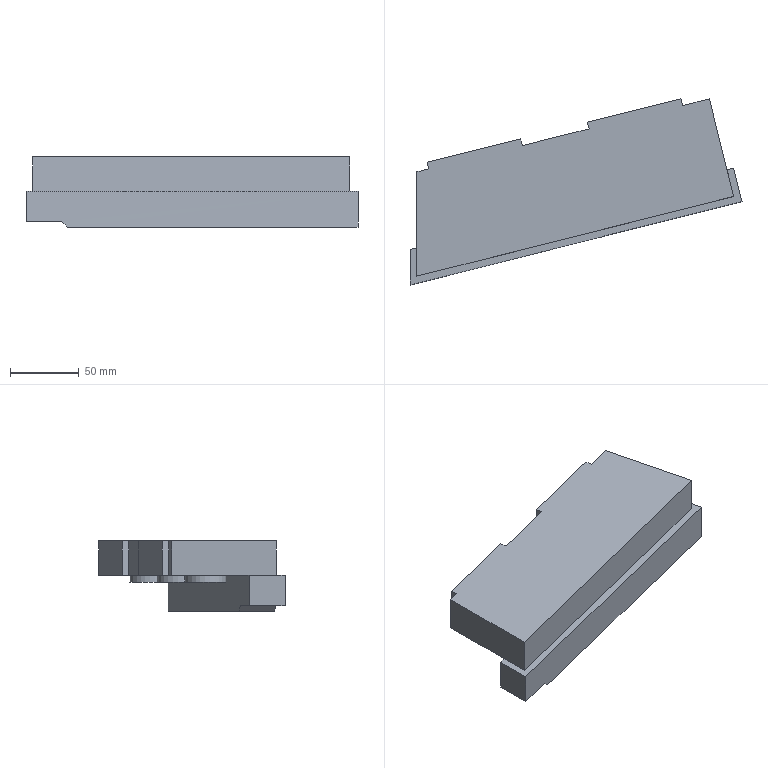Part | NX | features solid 2 | 1 solid | 32 faces | box 241.149 x 135.184 x 51 mm | volume 609918 mm3 | plane 24 | cylinder 5 | spline 3 | commonest cylinder face diameters 30 x5
STEP:
#1=CARTESIAN_POINT('',(-290.,474.207,-2.));
#2=VERTEX_POINT('',#1);
#3=CARTESIAN_POINT('',(-290.,499.994,-2.));
#4=VERTEX_POINT('',#3);
#5=CARTESIAN_POINT('',(-290.,600.,-2.));
#6=DIRECTION('',(0.,1.,0.));
#7=VECTOR('',#6,1000.);
#8=LINE('',#5,#7);
#9=EDGE_CURVE('',#2,#4,#8,.T.);
#10=ORIENTED_EDGE('',*,*,#9,.F.);
#11=CARTESIAN_POINT('',(-290.,474.207,20.));
#12=VERTEX_POINT('',#11);
#13=CARTESIAN_POINT('',(-290.,474.207,7.));
#14=DIRECTION('',(0.,0.,-1.));
#15=VECTOR('',#14,1000.);
#16=LINE('',#13,#15);
#17=EDGE_CURVE('',#2,#12,#16,.F.);
#18=ORIENTED_EDGE('',*,*,#17,.T.);
#19=CARTESIAN_POINT('',(-290.,499.994,20.));
#20=VERTEX_POINT('',#19);
#21=CARTESIAN_POINT('',(-290.,359.461,20.));
#22=DIRECTION('',(0.,-1.,0.));
#23=VECTOR('',#22,1000.);
#24=LINE('',#21,#23);
#25=EDGE_CURVE('',#12,#20,#24,.F.);
#26=ORIENTED_EDGE('',*,*,#25,.T.);
#27=CARTESIAN_POINT('',(-290.,499.994,7.));
#28=DIRECTION('',(0.,0.,1.));
#29=VECTOR('',#28,1000.);
#30=LINE('',#27,#29);
#31=EDGE_CURVE('',#20,#4,#30,.F.);
#32=ORIENTED_EDGE('',*,*,#31,.T.);
#33=EDGE_LOOP('',(#10,#18,#26,#32));
#34=FACE_BOUND('',#33,.T.);
#35=CARTESIAN_POINT('',(-290.,600.,0.));
#36=DIRECTION('',(-1.,0.,0.));
#37=DIRECTION('',(0.,0.,1.));
#38=AXIS2_PLACEMENT_3D('',#35,#36,#37);
#39=PLANE('',#38);
#40=ADVANCED_FACE('',(#34),#39,.T.);
#41=CARTESIAN_POINT('',(-192.908,552.089,20.));
#42=VERTEX_POINT('',#41);
#43=CARTESIAN_POINT('',(-177.908,552.089,20.));
#44=DIRECTION('',(0.,0.,-1.));
#45=DIRECTION('',(-1.,0.,0.));
#46=AXIS2_PLACEMENT_3D('',#43,#44,#45);
#47=CIRCLE('',#46,15.);
#48=EDGE_CURVE('',#42,#42,#47,.T.);
#49=ORIENTED_EDGE('',*,*,#48,.F.);
#50=EDGE_LOOP('',(#49));
#51=FACE_BOUND('',#50,.T.);
#52=CARTESIAN_POINT('',(-242.908,552.089,20.));
#53=VERTEX_POINT('',#52);
#54=CARTESIAN_POINT('',(-227.908,552.089,20.));
#55=DIRECTION('',(0.,0.,-1.));
#56=DIRECTION('',(-1.,0.,0.));
#57=AXIS2_PLACEMENT_3D('',#54,#55,#56);
#58=CIRCLE('',#57,15.);
#59=EDGE_CURVE('',#53,#53,#58,.T.);
#60=ORIENTED_EDGE('',*,*,#59,.F.);
#61=EDGE_LOOP('',(#60));
#62=FACE_BOUND('',#61,.T.);
#63=CARTESIAN_POINT('',(-272.908,532.089,20.));
#64=VERTEX_POINT('',#63);
#65=CARTESIAN_POINT('',(-257.908,532.089,20.));
#66=DIRECTION('',(0.,0.,-1.));
#67=DIRECTION('',(-1.,0.,0.));
#68=AXIS2_PLACEMENT_3D('',#65,#66,#67);
#69=CIRCLE('',#68,15.);
#70=EDGE_CURVE('',#64,#64,#69,.T.);
#71=ORIENTED_EDGE('',*,*,#70,.F.);
#72=EDGE_LOOP('',(#71));
#73=FACE_BOUND('',#72,.T.);
#74=CARTESIAN_POINT('',(-147.908,572.089,20.));
#75=VERTEX_POINT('',#74);
#76=CARTESIAN_POINT('',(-132.908,572.089,20.));
#77=DIRECTION('',(0.,0.,-1.));
#78=DIRECTION('',(-1.,0.,0.));
#79=AXIS2_PLACEMENT_3D('',#76,#77,#78);
#80=CIRCLE('',#79,15.);
#81=EDGE_CURVE('',#75,#75,#80,.T.);
#82=ORIENTED_EDGE('',*,*,#81,.F.);
#83=EDGE_LOOP('',(#82));
#84=FACE_BOUND('',#83,.T.);
#85=CARTESIAN_POINT('',(-112.908,572.089,20.));
#86=VERTEX_POINT('',#85);
#87=CARTESIAN_POINT('',(-97.908,572.089,20.));
#88=DIRECTION('',(0.,0.,-1.));
#89=DIRECTION('',(-1.,0.,0.));
#90=AXIS2_PLACEMENT_3D('',#87,#88,#89);
#91=CIRCLE('',#90,15.);
#92=EDGE_CURVE('',#86,#86,#91,.T.);
#93=ORIENTED_EDGE('',*,*,#92,.F.);
#94=EDGE_LOOP('',(#93));
#95=FACE_BOUND('',#94,.T.);
#96=CARTESIAN_POINT('',(-285.,501.256,20.));
#97=VERTEX_POINT('',#96);
#98=CARTESIAN_POINT('',(-59.748,557.921,20.));
#99=VERTEX_POINT('',#98);
#100=CARTESIAN_POINT('',(-285.,501.256,20.));
#101=CARTESIAN_POINT('',(-266.232,505.989,20.));
#102=CARTESIAN_POINT('',(-228.669,515.351,20.));
#103=CARTESIAN_POINT('',(-153.588,534.251,20.));
#104=CARTESIAN_POINT('',(-97.288,548.469,20.));
#105=CARTESIAN_POINT('',(-59.748,557.921,20.));
#106=B_SPLINE_CURVE_WITH_KNOTS('',3,(#100,#101,#102,#103,#104,#105),.UNSPECIFIED.,.F.,.F.,(4,1,1,4),(0.4597,0.5177,0.5758,0.6919),.UNSPECIFIED.);
#107=EDGE_CURVE('',#97,#99,#106,.T.);
#108=ORIENTED_EDGE('',*,*,#107,.F.);
#109=CARTESIAN_POINT('',(-285.,556.415,20.));
#110=VERTEX_POINT('',#109);
#111=CARTESIAN_POINT('',(-285.,482.459,20.));
#112=DIRECTION('',(0.,-1.,0.));
#113=VECTOR('',#112,1000.);
#114=LINE('',#111,#113);
#115=EDGE_CURVE('',#97,#110,#114,.F.);
#116=ORIENTED_EDGE('',*,*,#115,.T.);
#117=CARTESIAN_POINT('',(-276.34,558.574,20.));
#118=VERTEX_POINT('',#117);
#119=CARTESIAN_POINT('',(-334.558,544.059,20.));
#120=DIRECTION('',(-0.9703,-0.2419,0.));
#121=VECTOR('',#120,1000.);
#122=LINE('',#119,#121);
#123=EDGE_CURVE('',#110,#118,#122,.F.);
#124=ORIENTED_EDGE('',*,*,#123,.T.);
#125=CARTESIAN_POINT('',(-277.549,563.426,20.));
#126=VERTEX_POINT('',#125);
#127=CARTESIAN_POINT('',(-246.318,438.164,20.));
#128=DIRECTION('',(0.2419,-0.9703,0.));
#129=VECTOR('',#128,1000.);
#130=LINE('',#127,#129);
#131=EDGE_CURVE('',#118,#126,#130,.F.);
#132=ORIENTED_EDGE('',*,*,#131,.T.);
#133=CARTESIAN_POINT('',(-209.629,580.36,20.));
#134=VERTEX_POINT('',#133);
#135=CARTESIAN_POINT('',(-335.767,548.911,20.));
#136=DIRECTION('',(0.9703,0.2419,0.));
#137=VECTOR('',#136,1000.);
#138=LINE('',#135,#137);
#139=EDGE_CURVE('',#126,#134,#138,.T.);
#140=ORIENTED_EDGE('',*,*,#139,.T.);
#141=CARTESIAN_POINT('',(-208.419,575.509,20.));
#142=VERTEX_POINT('',#141);
#143=CARTESIAN_POINT('',(-178.397,455.098,20.));
#144=DIRECTION('',(0.2419,-0.9703,0.));
#145=VECTOR('',#144,1000.);
#146=LINE('',#143,#145);
#147=EDGE_CURVE('',#142,#134,#146,.F.);
#148=ORIENTED_EDGE('',*,*,#147,.F.);
#149=CARTESIAN_POINT('',(-159.904,587.605,20.));
#150=VERTEX_POINT('',#149);
#151=CARTESIAN_POINT('',(-334.558,544.059,20.));
#152=DIRECTION('',(-0.9703,-0.2419,0.));
#153=VECTOR('',#152,1000.);
#154=LINE('',#151,#153);
#155=EDGE_CURVE('',#142,#150,#154,.F.);
#156=ORIENTED_EDGE('',*,*,#155,.T.);
#157=CARTESIAN_POINT('',(-161.114,592.457,20.));
#158=VERTEX_POINT('',#157);
#159=CARTESIAN_POINT('',(-159.904,587.605,20.));
#160=DIRECTION('',(-0.2419,0.9703,0.));
#161=VECTOR('',#160,1000.);
#162=LINE('',#159,#161);
#163=EDGE_CURVE('',#150,#158,#162,.T.);
#164=ORIENTED_EDGE('',*,*,#163,.T.);
#165=CARTESIAN_POINT('',(-93.193,609.391,20.));
#166=VERTEX_POINT('',#165);
#167=CARTESIAN_POINT('',(-132.005,599.714,20.));
#168=DIRECTION('',(0.9703,0.2419,0.));
#169=VECTOR('',#168,1000.);
#170=LINE('',#167,#169);
#171=EDGE_CURVE('',#158,#166,#170,.T.);
#172=ORIENTED_EDGE('',*,*,#171,.T.);
#173=CARTESIAN_POINT('',(-91.984,604.54,20.));
#174=VERTEX_POINT('',#173);
#175=CARTESIAN_POINT('',(-91.984,604.54,20.));
#176=DIRECTION('',(-0.2419,0.9703,0.));
#177=VECTOR('',#176,1000.);
#178=LINE('',#175,#177);
#179=EDGE_CURVE('',#174,#166,#178,.T.);
#180=ORIENTED_EDGE('',*,*,#179,.F.);
#181=CARTESIAN_POINT('',(-72.578,609.378,20.));
#182=VERTEX_POINT('',#181);
#183=CARTESIAN_POINT('',(-334.558,544.059,20.));
#184=DIRECTION('',(-0.9703,-0.2419,0.));
#185=VECTOR('',#184,1000.);
#186=LINE('',#183,#185);
#187=EDGE_CURVE('',#174,#182,#186,.F.);
#188=ORIENTED_EDGE('',*,*,#187,.T.);
#189=CARTESIAN_POINT('',(-54.912,538.526,20.));
#190=DIRECTION('',(0.2419,-0.9703,0.));
#191=VECTOR('',#190,1000.);
#192=LINE('',#189,#191);
#193=EDGE_CURVE('',#99,#182,#192,.F.);
#194=ORIENTED_EDGE('',*,*,#193,.F.);
#195=EDGE_LOOP('',(#108,#116,#124,#132,#140,#148,#156,#164,#172,#180,#188,#194));
#196=FACE_BOUND('',#195,.T.);
#197=CARTESIAN_POINT('',(-561.977,359.461,20.));
#198=DIRECTION('',(0.,0.,-1.));
#199=DIRECTION('',(-1.,0.,0.));
#200=AXIS2_PLACEMENT_3D('',#197,#198,#199);
#201=PLANE('',#200);
#202=ADVANCED_FACE('',(#51,#62,#73,#84,#95,#196),#201,.T.);
#203=CARTESIAN_POINT('',(-285.,480.629,45.));
#204=VERTEX_POINT('',#203);
#205=CARTESIAN_POINT('',(-285.,556.415,45.));
#206=VERTEX_POINT('',#205);
#207=CARTESIAN_POINT('',(-285.,-794.984,45.));
#208=DIRECTION('',(0.,1.,0.));
#209=VECTOR('',#208,1000.);
#210=LINE('',#207,#209);
#211=EDGE_CURVE('',#204,#206,#210,.T.);
#212=ORIENTED_EDGE('',*,*,#211,.F.);
#213=CARTESIAN_POINT('',(-54.91,538.515,45.));
#214=VERTEX_POINT('',#213);
#215=CARTESIAN_POINT('',(-285.,480.629,45.));
#216=CARTESIAN_POINT('',(-265.83,485.471,45.));
#217=CARTESIAN_POINT('',(-227.462,495.038,45.));
#218=CARTESIAN_POINT('',(-150.765,514.332,45.));
#219=CARTESIAN_POINT('',(-93.256,528.86,45.));
#220=CARTESIAN_POINT('',(-54.91,538.515,45.));
#221=B_SPLINE_CURVE_WITH_KNOTS('',3,(#215,#216,#217,#218,#219,#220),.UNSPECIFIED.,.F.,.F.,(4,1,1,4),(0.02774,0.08706,0.1464,0.265),.UNSPECIFIED.);
#222=EDGE_CURVE('',#204,#214,#221,.T.);
#223=ORIENTED_EDGE('',*,*,#222,.T.);
#224=CARTESIAN_POINT('',(-72.578,609.378,45.));
#225=VERTEX_POINT('',#224);
#226=CARTESIAN_POINT('',(-54.912,538.526,45.));
#227=DIRECTION('',(-0.2419,0.9703,0.));
#228=VECTOR('',#227,1000.);
#229=LINE('',#226,#228);
#230=EDGE_CURVE('',#214,#225,#229,.T.);
#231=ORIENTED_EDGE('',*,*,#230,.T.);
#232=CARTESIAN_POINT('',(-91.984,604.54,45.));
#233=VERTEX_POINT('',#232);
#234=CARTESIAN_POINT('',(-334.558,544.059,45.));
#235=DIRECTION('',(0.9703,0.2419,0.));
#236=VECTOR('',#235,1000.);
#237=LINE('',#234,#236);
#238=EDGE_CURVE('',#233,#225,#237,.T.);
#239=ORIENTED_EDGE('',*,*,#238,.F.);
#240=CARTESIAN_POINT('',(-93.193,609.391,45.));
#241=VERTEX_POINT('',#240);
#242=CARTESIAN_POINT('',(-91.984,604.54,45.));
#243=DIRECTION('',(-0.2419,0.9703,0.));
#244=VECTOR('',#243,1000.);
#245=LINE('',#242,#244);
#246=EDGE_CURVE('',#233,#241,#245,.T.);
#247=ORIENTED_EDGE('',*,*,#246,.T.);
#248=CARTESIAN_POINT('',(-161.114,592.457,45.));
#249=VERTEX_POINT('',#248);
#250=CARTESIAN_POINT('',(-132.005,599.714,45.));
#251=DIRECTION('',(0.9703,0.2419,0.));
#252=VECTOR('',#251,1000.);
#253=LINE('',#250,#252);
#254=EDGE_CURVE('',#249,#241,#253,.T.);
#255=ORIENTED_EDGE('',*,*,#254,.F.);
#256=CARTESIAN_POINT('',(-159.904,587.605,45.));
#257=VERTEX_POINT('',#256);
#258=CARTESIAN_POINT('',(-159.904,587.605,45.));
#259=DIRECTION('',(-0.2419,0.9703,0.));
#260=VECTOR('',#259,1000.);
#261=LINE('',#258,#260);
#262=EDGE_CURVE('',#257,#249,#261,.T.);
#263=ORIENTED_EDGE('',*,*,#262,.F.);
#264=CARTESIAN_POINT('',(-208.419,575.509,45.));
#265=VERTEX_POINT('',#264);
#266=CARTESIAN_POINT('',(-334.558,544.059,45.));
#267=DIRECTION('',(0.9703,0.2419,0.));
#268=VECTOR('',#267,1000.);
#269=LINE('',#266,#268);
#270=EDGE_CURVE('',#265,#257,#269,.T.);
#271=ORIENTED_EDGE('',*,*,#270,.F.);
#272=CARTESIAN_POINT('',(-209.629,580.36,45.));
#273=VERTEX_POINT('',#272);
#274=CARTESIAN_POINT('',(120.792,-744.886,45.));
#275=DIRECTION('',(-0.2419,0.9703,0.));
#276=VECTOR('',#275,1000.);
#277=LINE('',#274,#276);
#278=EDGE_CURVE('',#265,#273,#277,.T.);
#279=ORIENTED_EDGE('',*,*,#278,.T.);
#280=CARTESIAN_POINT('',(-277.549,563.426,45.));
#281=VERTEX_POINT('',#280);
#282=CARTESIAN_POINT('',(-335.767,548.911,45.));
#283=DIRECTION('',(0.9703,0.2419,0.));
#284=VECTOR('',#283,1000.);
#285=LINE('',#282,#284);
#286=EDGE_CURVE('',#281,#273,#285,.T.);
#287=ORIENTED_EDGE('',*,*,#286,.F.);
#288=CARTESIAN_POINT('',(-276.34,558.574,45.));
#289=VERTEX_POINT('',#288);
#290=CARTESIAN_POINT('',(52.872,-761.821,45.));
#291=DIRECTION('',(-0.2419,0.9703,0.));
#292=VECTOR('',#291,1000.);
#293=LINE('',#290,#292);
#294=EDGE_CURVE('',#289,#281,#293,.T.);
#295=ORIENTED_EDGE('',*,*,#294,.F.);
#296=CARTESIAN_POINT('',(-334.558,544.059,45.));
#297=DIRECTION('',(0.9703,0.2419,0.));
#298=VECTOR('',#297,1000.);
#299=LINE('',#296,#298);
#300=EDGE_CURVE('',#206,#289,#299,.T.);
#301=ORIENTED_EDGE('',*,*,#300,.F.);
#302=EDGE_LOOP('',(#212,#223,#231,#239,#247,#255,#263,#271,#279,#287,#295,#301));
#303=FACE_BOUND('',#302,.T.);
#304=CARTESIAN_POINT('',(-80.139,-794.984,45.));
#305=DIRECTION('',(0.,0.,1.));
#306=DIRECTION('',(1.,0.,0.));
#307=AXIS2_PLACEMENT_3D('',#304,#305,#306);
#308=PLANE('',#307);
#309=ADVANCED_FACE('',(#303),#308,.T.);
#310=CARTESIAN_POINT('',(-260.,481.763,-6.));
#311=VERTEX_POINT('',#310);
#312=CARTESIAN_POINT('',(-48.851,534.884,-6.));
#313=VERTEX_POINT('',#312);
#314=CARTESIAN_POINT('',(-48.851,534.884,-6.));
#315=CARTESIAN_POINT('',(-84.041,526.025,-6.));
#316=CARTESIAN_POINT('',(-154.403,508.24,-6.));
#317=CARTESIAN_POINT('',(-224.801,490.59,-6.));
#318=CARTESIAN_POINT('',(-260.,481.763,-6.));
#319=B_SPLINE_CURVE_WITH_KNOTS('',3,(#314,#315,#316,#317,#318),.UNSPECIFIED.,.F.,.F.,(4,1,4),(0.4841,0.5929,0.7018),.UNSPECIFIED.);
#320=EDGE_CURVE('',#311,#313,#319,.F.);
#321=ORIENTED_EDGE('',*,*,#320,.F.);
#322=CARTESIAN_POINT('',(-260.,507.536,-6.));
#323=VERTEX_POINT('',#322);
#324=CARTESIAN_POINT('',(-260.,-794.984,-6.));
#325=DIRECTION('',(0.,1.,0.));
#326=VECTOR('',#325,1000.);
#327=LINE('',#324,#326);
#328=EDGE_CURVE('',#311,#323,#327,.T.);
#329=ORIENTED_EDGE('',*,*,#328,.T.);
#330=CARTESIAN_POINT('',(-54.899,559.142,-6.));
#331=VERTEX_POINT('',#330);
#332=CARTESIAN_POINT('',(-260.,507.536,-6.));
#333=CARTESIAN_POINT('',(-191.614,524.661,-6.));
#334=CARTESIAN_POINT('',(-123.264,541.93,-6.));
#335=CARTESIAN_POINT('',(-54.899,559.142,-6.));
#336=B_SPLINE_CURVE_WITH_KNOTS('',3,(#332,#333,#334,#335),.UNSPECIFIED.,.F.,.F.,(4,4),(0.4856,0.6971),.UNSPECIFIED.);
#337=EDGE_CURVE('',#323,#331,#336,.T.);
#338=ORIENTED_EDGE('',*,*,#337,.T.);
#339=CARTESIAN_POINT('',(563.408,-1920.754,-6.));
#340=DIRECTION('',(-0.2419,0.9703,0.));
#341=VECTOR('',#340,1000.);
#342=LINE('',#339,#341);
#343=EDGE_CURVE('',#313,#331,#342,.T.);
#344=ORIENTED_EDGE('',*,*,#343,.F.);
#345=EDGE_LOOP('',(#321,#329,#338,#344));
#346=FACE_BOUND('',#345,.T.);
#347=CARTESIAN_POINT('',(-80.139,-794.984,-6.));
#348=DIRECTION('',(0.,0.,1.));
#349=DIRECTION('',(1.,0.,0.));
#350=AXIS2_PLACEMENT_3D('',#347,#348,#349);
#351=PLANE('',#350);
#352=ADVANCED_FACE('',(#346),#351,.F.);
#353=CARTESIAN_POINT('',(-264.,480.76,-2.));
#354=VERTEX_POINT('',#353);
#355=CARTESIAN_POINT('',(-290.,474.207,-2.));
#356=CARTESIAN_POINT('',(-281.336,476.401,-2.));
#357=CARTESIAN_POINT('',(-272.669,478.584,-2.));
#358=CARTESIAN_POINT('',(-264.,480.76,-2.));
#359=B_SPLINE_CURVE_WITH_KNOTS('',3,(#355,#356,#357,#358),.UNSPECIFIED.,.F.,.F.,(4,4),(0.1598,0.1865),.UNSPECIFIED.);
#360=EDGE_CURVE('',#2,#354,#359,.T.);
#361=ORIENTED_EDGE('',*,*,#360,.T.);
#362=CARTESIAN_POINT('',(-264.,480.76,-2.));
#363=CARTESIAN_POINT('',(-262.667,481.095,-3.333));
#364=CARTESIAN_POINT('',(-261.333,481.429,-4.667));
#365=CARTESIAN_POINT('',(-260.,481.763,-6.));
#366=B_SPLINE_CURVE_WITH_KNOTS('',3,(#362,#363,#364,#365),.UNSPECIFIED.,.F.,.F.,(4,4),(0.,0.005745),.UNSPECIFIED.);
#367=EDGE_CURVE('',#354,#311,#366,.T.);
#368=ORIENTED_EDGE('',*,*,#367,.T.);
#369=ORIENTED_EDGE('',*,*,#320,.T.);
#370=CARTESIAN_POINT('',(-48.851,534.884,20.));
#371=VERTEX_POINT('',#370);
#372=CARTESIAN_POINT('',(-48.851,534.884,30.));
#373=DIRECTION('',(0.,0.,-1.));
#374=VECTOR('',#373,1000.);
#375=LINE('',#372,#374);
#376=EDGE_CURVE('',#371,#313,#375,.T.);
#377=ORIENTED_EDGE('',*,*,#376,.F.);
#378=CARTESIAN_POINT('',(-48.851,534.884,20.));
#379=CARTESIAN_POINT('',(-89.041,524.766,20.));
#380=CARTESIAN_POINT('',(-149.312,509.537,20.));
#381=CARTESIAN_POINT('',(-229.699,489.326,20.));
#382=CARTESIAN_POINT('',(-269.912,479.293,20.));
#383=CARTESIAN_POINT('',(-290.,474.207,20.));
#384=B_SPLINE_CURVE_WITH_KNOTS('',3,(#378,#379,#380,#381,#382,#383),.UNSPECIFIED.,.F.,.F.,(4,1,1,4),(0.4669,0.5913,0.6534,0.7156),.UNSPECIFIED.);
#385=EDGE_CURVE('',#12,#371,#384,.F.);
#386=ORIENTED_EDGE('',*,*,#385,.F.);
#387=ORIENTED_EDGE('',*,*,#17,.F.);
#388=EDGE_LOOP('',(#361,#368,#369,#377,#386,#387));
#389=FACE_BOUND('',#388,.T.);
#390=CARTESIAN_POINT('',(-290.,474.207,20.));
#391=CARTESIAN_POINT('',(-290.,474.207,-6.));
#392=CARTESIAN_POINT('',(-269.911,479.293,20.));
#393=CARTESIAN_POINT('',(-269.911,479.293,-6.));
#394=CARTESIAN_POINT('',(-229.7,489.326,20.));
#395=CARTESIAN_POINT('',(-229.7,489.326,-6.));
#396=CARTESIAN_POINT('',(-149.313,509.536,20.));
#397=CARTESIAN_POINT('',(-149.313,509.536,-6.));
#398=CARTESIAN_POINT('',(-89.041,524.766,20.));
#399=CARTESIAN_POINT('',(-89.041,524.766,-6.));
#400=CARTESIAN_POINT('',(-48.851,534.884,20.));
#401=CARTESIAN_POINT('',(-48.851,534.884,-6.));
#402=B_SPLINE_SURFACE_WITH_KNOTS('',3,1,((#390,#391),(#392,#393),(#394,#395),(#396,#397),(#398,#399),(#400,#401)),.SURF_OF_LINEAR_EXTRUSION.,.F.,.F.,.F.,(4,1,1,4),(2,2),(0.5601,0.6132,0.6663,0.7724),(0.,1.),.UNSPECIFIED.);
#403=ADVANCED_FACE('',(#389),#402,.F.);
#404=CARTESIAN_POINT('',(-285.,480.629,20.));
#405=VERTEX_POINT('',#404);
#406=CARTESIAN_POINT('',(-54.91,538.515,20.));
#407=VERTEX_POINT('',#406);
#408=CARTESIAN_POINT('',(-285.,480.629,20.));
#409=CARTESIAN_POINT('',(-265.83,485.471,20.));
#410=CARTESIAN_POINT('',(-227.462,495.038,20.));
#411=CARTESIAN_POINT('',(-150.765,514.332,20.));
#412=CARTESIAN_POINT('',(-93.256,528.86,20.));
#413=CARTESIAN_POINT('',(-54.91,538.515,20.));
#414=B_SPLINE_CURVE_WITH_KNOTS('',3,(#408,#409,#410,#411,#412,#413),.UNSPECIFIED.,.F.,.F.,(4,1,1,4),(1.119,1.178,1.237,1.356),.UNSPECIFIED.);
#415=EDGE_CURVE('',#405,#407,#414,.T.);
#416=ORIENTED_EDGE('',*,*,#415,.F.);
#417=CARTESIAN_POINT('',(-285.,482.459,20.));
#418=DIRECTION('',(0.,-1.,0.));
#419=VECTOR('',#418,1000.);
#420=LINE('',#417,#419);
#421=EDGE_CURVE('',#405,#97,#420,.F.);
#422=ORIENTED_EDGE('',*,*,#421,.T.);
#423=CARTESIAN_POINT('',(-290.,499.994,20.));
#424=CARTESIAN_POINT('',(-288.333,500.415,20.));
#425=CARTESIAN_POINT('',(-286.667,500.836,20.));
#426=CARTESIAN_POINT('',(-285.,501.256,20.));
#427=B_SPLINE_CURVE_WITH_KNOTS('',3,(#423,#424,#425,#426),.UNSPECIFIED.,.F.,.F.,(4,4),(0.4545,0.4597),.UNSPECIFIED.);
#428=EDGE_CURVE('',#20,#97,#427,.T.);
#429=ORIENTED_EDGE('',*,*,#428,.F.);
#430=ORIENTED_EDGE('',*,*,#25,.F.);
#431=ORIENTED_EDGE('',*,*,#385,.T.);
#432=CARTESIAN_POINT('',(-54.899,559.142,20.));
#433=VERTEX_POINT('',#432);
#434=CARTESIAN_POINT('',(-48.691,534.243,20.));
#435=DIRECTION('',(0.2419,-0.9703,0.));
#436=VECTOR('',#435,1000.);
#437=LINE('',#434,#436);
#438=EDGE_CURVE('',#371,#433,#437,.F.);
#439=ORIENTED_EDGE('',*,*,#438,.T.);
#440=CARTESIAN_POINT('',(-54.899,559.142,20.));
#441=CARTESIAN_POINT('',(-56.516,558.735,20.));
#442=CARTESIAN_POINT('',(-58.132,558.328,20.));
#443=CARTESIAN_POINT('',(-59.748,557.921,20.));
#444=B_SPLINE_CURVE_WITH_KNOTS('',3,(#440,#441,#442,#443),.UNSPECIFIED.,.F.,.F.,(4,4),(0.,0.005),.UNSPECIFIED.);
#445=EDGE_CURVE('',#99,#433,#444,.F.);
#446=ORIENTED_EDGE('',*,*,#445,.F.);
#447=CARTESIAN_POINT('',(-53.543,533.033,20.));
#448=DIRECTION('',(0.2419,-0.9703,0.));
#449=VECTOR('',#448,1000.);
#450=LINE('',#447,#449);
#451=EDGE_CURVE('',#407,#99,#450,.F.);
#452=ORIENTED_EDGE('',*,*,#451,.F.);
#453=EDGE_LOOP('',(#416,#422,#429,#430,#431,#439,#446,#452));
#454=FACE_BOUND('',#453,.T.);
#455=CARTESIAN_POINT('',(-561.977,359.461,20.));
#456=DIRECTION('',(0.,0.,1.));
#457=DIRECTION('',(1.,0.,0.));
#458=AXIS2_PLACEMENT_3D('',#455,#456,#457);
#459=PLANE('',#458);
#460=ADVANCED_FACE('',(#454),#459,.T.);
#461=CARTESIAN_POINT('',(-285.,556.415,70.));
#462=DIRECTION('',(0.,0.,-1.));
#463=VECTOR('',#462,1000.);
#464=LINE('',#461,#463);
#465=EDGE_CURVE('',#206,#110,#464,.T.);
#466=ORIENTED_EDGE('',*,*,#465,.F.);
#467=ORIENTED_EDGE('',*,*,#300,.T.);
#468=CARTESIAN_POINT('',(-276.34,558.574,70.));
#469=DIRECTION('',(0.,0.,-1.));
#470=VECTOR('',#469,1000.);
#471=LINE('',#468,#470);
#472=EDGE_CURVE('',#289,#118,#471,.T.);
#473=ORIENTED_EDGE('',*,*,#472,.T.);
#474=ORIENTED_EDGE('',*,*,#123,.F.);
#475=EDGE_LOOP('',(#466,#467,#473,#474));
#476=FACE_BOUND('',#475,.T.);
#477=CARTESIAN_POINT('',(-334.558,544.059,70.));
#478=DIRECTION('',(-0.2419,0.9703,0.));
#479=DIRECTION('',(-0.9703,-0.2419,0.));
#480=AXIS2_PLACEMENT_3D('',#477,#478,#479);
#481=PLANE('',#480);
#482=ADVANCED_FACE('',(#476),#481,.T.);
#483=ORIENTED_EDGE('',*,*,#222,.F.);
#484=CARTESIAN_POINT('',(-285.,480.629,32.5));
#485=DIRECTION('',(0.,0.,-1.));
#486=VECTOR('',#485,1000.);
#487=LINE('',#484,#486);
#488=EDGE_CURVE('',#204,#405,#487,.T.);
#489=ORIENTED_EDGE('',*,*,#488,.T.);
#490=ORIENTED_EDGE('',*,*,#415,.T.);
#491=CARTESIAN_POINT('',(-54.91,538.515,42.5));
#492=DIRECTION('',(0.,0.,-1.));
#493=VECTOR('',#492,1000.);
#494=LINE('',#491,#493);
#495=EDGE_CURVE('',#214,#407,#494,.T.);
#496=ORIENTED_EDGE('',*,*,#495,.F.);
#497=EDGE_LOOP('',(#483,#489,#490,#496));
#498=FACE_BOUND('',#497,.T.);
#499=CARTESIAN_POINT('',(-285.,480.629,45.));
#500=CARTESIAN_POINT('',(-285.,480.629,20.));
#501=CARTESIAN_POINT('',(-265.823,485.473,45.));
#502=CARTESIAN_POINT('',(-265.823,485.473,20.));
#503=CARTESIAN_POINT('',(-227.448,495.042,45.));
#504=CARTESIAN_POINT('',(-227.448,495.042,20.));
#505=CARTESIAN_POINT('',(-150.771,514.33,45.));
#506=CARTESIAN_POINT('',(-150.771,514.33,20.));
#507=CARTESIAN_POINT('',(-93.256,528.86,45.));
#508=CARTESIAN_POINT('',(-93.256,528.86,20.));
#509=CARTESIAN_POINT('',(-54.91,538.515,45.));
#510=CARTESIAN_POINT('',(-54.91,538.515,20.));
#511=B_SPLINE_SURFACE_WITH_KNOTS('',3,1,((#499,#500),(#501,#502),(#503,#504),(#505,#506),(#507,#508),(#509,#510)),.SURF_OF_LINEAR_EXTRUSION.,.F.,.F.,.F.,(4,1,1,4),(2,2),(0.1028,0.3225,0.5422,0.9815),(0.,1.),.UNSPECIFIED.);
#512=ADVANCED_FACE('',(#498),#511,.F.);
#513=ORIENTED_EDGE('',*,*,#337,.F.);
#514=CARTESIAN_POINT('',(-264.,506.534,-2.));
#515=VERTEX_POINT('',#514);
#516=CARTESIAN_POINT('',(-260.,507.536,-6.));
#517=CARTESIAN_POINT('',(-261.333,507.202,-4.667));
#518=CARTESIAN_POINT('',(-262.667,506.868,-3.333));
#519=CARTESIAN_POINT('',(-264.,506.534,-2.));
#520=B_SPLINE_CURVE_WITH_KNOTS('',3,(#516,#517,#518,#519),.UNSPECIFIED.,.F.,.F.,(4,4),(0.,0.005745),.UNSPECIFIED.);
#521=EDGE_CURVE('',#323,#515,#520,.T.);
#522=ORIENTED_EDGE('',*,*,#521,.T.);
#523=CARTESIAN_POINT('',(-264.,506.534,-2.));
#524=CARTESIAN_POINT('',(-272.669,504.362,-2.));
#525=CARTESIAN_POINT('',(-281.336,502.183,-2.));
#526=CARTESIAN_POINT('',(-290.,499.994,-2.));
#527=B_SPLINE_CURVE_WITH_KNOTS('',3,(#523,#524,#525,#526),.UNSPECIFIED.,.F.,.F.,(4,4),(0.002062,0.02887),.UNSPECIFIED.);
#528=EDGE_CURVE('',#515,#4,#527,.T.);
#529=ORIENTED_EDGE('',*,*,#528,.T.);
#530=ORIENTED_EDGE('',*,*,#31,.F.);
#531=ORIENTED_EDGE('',*,*,#428,.T.);
#532=ORIENTED_EDGE('',*,*,#107,.T.);
#533=ORIENTED_EDGE('',*,*,#445,.T.);
#534=CARTESIAN_POINT('',(-54.899,559.142,9.5));
#535=DIRECTION('',(0.,0.,1.));
#536=VECTOR('',#535,1000.);
#537=LINE('',#534,#536);
#538=EDGE_CURVE('',#331,#433,#537,.T.);
#539=ORIENTED_EDGE('',*,*,#538,.F.);
#540=EDGE_LOOP('',(#513,#522,#529,#530,#531,#532,#533,#539));
#541=FACE_BOUND('',#540,.T.);
#542=CARTESIAN_POINT('',(-290.,499.994,-6.));
#543=CARTESIAN_POINT('',(-290.,499.994,20.));
#544=CARTESIAN_POINT('',(-270.373,504.952,-6.));
#545=CARTESIAN_POINT('',(-270.373,504.952,20.));
#546=CARTESIAN_POINT('',(-231.142,514.732,-6.));
#547=CARTESIAN_POINT('',(-231.142,514.732,20.));
#548=CARTESIAN_POINT('',(-152.878,534.427,-6.));
#549=CARTESIAN_POINT('',(-152.878,534.427,20.));
#550=CARTESIAN_POINT('',(-94.078,549.278,-6.));
#551=CARTESIAN_POINT('',(-94.078,549.278,20.));
#552=CARTESIAN_POINT('',(-54.899,559.142,-6.));
#553=CARTESIAN_POINT('',(-54.899,559.142,20.));
#554=B_SPLINE_SURFACE_WITH_KNOTS('',3,1,((#542,#543),(#544,#545),(#546,#547),(#548,#549),(#550,#551),(#552,#553)),.SURF_OF_LINEAR_EXTRUSION.,.F.,.F.,.F.,(4,1,1,4),(2,2),(0.1024,0.3269,0.5513,1.),(0.,1.),.UNSPECIFIED.);
#555=ADVANCED_FACE('',(#541),#554,.F.);
#556=ORIENTED_EDGE('',*,*,#270,.T.);
#557=CARTESIAN_POINT('',(-159.904,587.605,45.));
#558=DIRECTION('',(0.,0.,1.));
#559=VECTOR('',#558,1000.);
#560=LINE('',#557,#559);
#561=EDGE_CURVE('',#257,#150,#560,.F.);
#562=ORIENTED_EDGE('',*,*,#561,.T.);
#563=ORIENTED_EDGE('',*,*,#155,.F.);
#564=CARTESIAN_POINT('',(-208.419,575.509,70.));
#565=DIRECTION('',(0.,0.,-1.));
#566=VECTOR('',#565,1000.);
#567=LINE('',#564,#566);
#568=EDGE_CURVE('',#265,#142,#567,.T.);
#569=ORIENTED_EDGE('',*,*,#568,.F.);
#570=EDGE_LOOP('',(#556,#562,#563,#569));
#571=FACE_BOUND('',#570,.T.);
#572=CARTESIAN_POINT('',(-334.558,544.059,70.));
#573=DIRECTION('',(-0.2419,0.9703,0.));
#574=DIRECTION('',(-0.9703,-0.2419,0.));
#575=AXIS2_PLACEMENT_3D('',#572,#573,#574);
#576=PLANE('',#575);
#577=ADVANCED_FACE('',(#571),#576,.T.);
#578=CARTESIAN_POINT('',(-91.984,604.54,45.));
#579=DIRECTION('',(0.,0.,-1.));
#580=VECTOR('',#579,1000.);
#581=LINE('',#578,#580);
#582=EDGE_CURVE('',#233,#174,#581,.T.);
#583=ORIENTED_EDGE('',*,*,#582,.F.);
#584=ORIENTED_EDGE('',*,*,#238,.T.);
#585=CARTESIAN_POINT('',(-72.578,609.378,70.));
#586=DIRECTION('',(0.,0.,-1.));
#587=VECTOR('',#586,1000.);
#588=LINE('',#585,#587);
#589=EDGE_CURVE('',#225,#182,#588,.T.);
#590=ORIENTED_EDGE('',*,*,#589,.T.);
#591=ORIENTED_EDGE('',*,*,#187,.F.);
#592=EDGE_LOOP('',(#583,#584,#590,#591));
#593=FACE_BOUND('',#592,.T.);
#594=CARTESIAN_POINT('',(-334.558,544.059,70.));
#595=DIRECTION('',(-0.2419,0.9703,0.));
#596=DIRECTION('',(-0.9703,-0.2419,0.));
#597=AXIS2_PLACEMENT_3D('',#594,#595,#596);
#598=PLANE('',#597);
#599=ADVANCED_FACE('',(#593),#598,.T.);
#600=ORIENTED_EDGE('',*,*,#343,.T.);
#601=ORIENTED_EDGE('',*,*,#538,.T.);
#602=ORIENTED_EDGE('',*,*,#438,.F.);
#603=ORIENTED_EDGE('',*,*,#376,.T.);
#604=EDGE_LOOP('',(#600,#601,#602,#603));
#605=FACE_BOUND('',#604,.T.);
#606=CARTESIAN_POINT('',(563.408,-1920.754,70.));
#607=DIRECTION('',(-0.9703,-0.2419,0.));
#608=DIRECTION('',(0.2419,-0.9703,0.));
#609=AXIS2_PLACEMENT_3D('',#606,#607,#608);
#610=PLANE('',#609);
#611=ADVANCED_FACE('',(#605),#610,.F.);
#612=ORIENTED_EDGE('',*,*,#451,.T.);
#613=ORIENTED_EDGE('',*,*,#193,.T.);
#614=ORIENTED_EDGE('',*,*,#589,.F.);
#615=ORIENTED_EDGE('',*,*,#230,.F.);
#616=ORIENTED_EDGE('',*,*,#495,.T.);
#617=EDGE_LOOP('',(#612,#613,#614,#615,#616));
#618=FACE_BOUND('',#617,.T.);
#619=CARTESIAN_POINT('',(-54.912,538.526,70.));
#620=DIRECTION('',(-0.9703,-0.2419,0.));
#621=DIRECTION('',(0.2419,-0.9703,0.));
#622=AXIS2_PLACEMENT_3D('',#619,#620,#621);
#623=PLANE('',#622);
#624=ADVANCED_FACE('',(#618),#623,.F.);
#625=CARTESIAN_POINT('',(-209.629,580.36,45.));
#626=DIRECTION('',(0.,0.,-1.));
#627=VECTOR('',#626,1000.);
#628=LINE('',#625,#627);
#629=EDGE_CURVE('',#273,#134,#628,.T.);
#630=ORIENTED_EDGE('',*,*,#629,.F.);
#631=ORIENTED_EDGE('',*,*,#278,.F.);
#632=ORIENTED_EDGE('',*,*,#568,.T.);
#633=ORIENTED_EDGE('',*,*,#147,.T.);
#634=EDGE_LOOP('',(#630,#631,#632,#633));
#635=FACE_BOUND('',#634,.T.);
#636=CARTESIAN_POINT('',(-208.419,575.509,45.));
#637=DIRECTION('',(0.9703,0.2419,0.));
#638=DIRECTION('',(-0.2419,0.9703,0.));
#639=AXIS2_PLACEMENT_3D('',#636,#637,#638);
#640=PLANE('',#639);
#641=ADVANCED_FACE('',(#635),#640,.T.);
#642=CARTESIAN_POINT('',(-277.549,563.426,45.));
#643=DIRECTION('',(0.,0.,-1.));
#644=VECTOR('',#643,1000.);
#645=LINE('',#642,#644);
#646=EDGE_CURVE('',#281,#126,#645,.T.);
#647=ORIENTED_EDGE('',*,*,#646,.T.);
#648=ORIENTED_EDGE('',*,*,#131,.F.);
#649=ORIENTED_EDGE('',*,*,#472,.F.);
#650=ORIENTED_EDGE('',*,*,#294,.T.);
#651=EDGE_LOOP('',(#647,#648,#649,#650));
#652=FACE_BOUND('',#651,.T.);
#653=CARTESIAN_POINT('',(-276.34,558.574,45.));
#654=DIRECTION('',(0.9703,0.2419,0.));
#655=DIRECTION('',(-0.2419,0.9703,0.));
#656=AXIS2_PLACEMENT_3D('',#653,#654,#655);
#657=PLANE('',#656);
#658=ADVANCED_FACE('',(#652),#657,.F.);
#659=ORIENTED_EDGE('',*,*,#629,.T.);
#660=ORIENTED_EDGE('',*,*,#139,.F.);
#661=ORIENTED_EDGE('',*,*,#646,.F.);
#662=ORIENTED_EDGE('',*,*,#286,.T.);
#663=EDGE_LOOP('',(#659,#660,#661,#662));
#664=FACE_BOUND('',#663,.T.);
#665=CARTESIAN_POINT('',(-335.767,548.911,45.));
#666=DIRECTION('',(0.2419,-0.9703,0.));
#667=DIRECTION('',(0.,0.,-1.));
#668=AXIS2_PLACEMENT_3D('',#665,#666,#667);
#669=PLANE('',#668);
#670=ADVANCED_FACE('',(#664),#669,.F.);
#671=CARTESIAN_POINT('',(-93.193,609.391,45.));
#672=DIRECTION('',(0.,0.,-1.));
#673=VECTOR('',#672,1000.);
#674=LINE('',#671,#673);
#675=EDGE_CURVE('',#241,#166,#674,.T.);
#676=ORIENTED_EDGE('',*,*,#675,.F.);
#677=ORIENTED_EDGE('',*,*,#246,.F.);
#678=ORIENTED_EDGE('',*,*,#582,.T.);
#679=ORIENTED_EDGE('',*,*,#179,.T.);
#680=EDGE_LOOP('',(#676,#677,#678,#679));
#681=FACE_BOUND('',#680,.T.);
#682=CARTESIAN_POINT('',(-91.984,604.54,45.));
#683=DIRECTION('',(0.9703,0.2419,0.));
#684=DIRECTION('',(-0.2419,0.9703,0.));
#685=AXIS2_PLACEMENT_3D('',#682,#683,#684);
#686=PLANE('',#685);
#687=ADVANCED_FACE('',(#681),#686,.T.);
#688=CARTESIAN_POINT('',(-161.114,592.457,45.));
#689=DIRECTION('',(0.,0.,1.));
#690=VECTOR('',#689,1000.);
#691=LINE('',#688,#690);
#692=EDGE_CURVE('',#249,#158,#691,.F.);
#693=ORIENTED_EDGE('',*,*,#692,.T.);
#694=ORIENTED_EDGE('',*,*,#163,.F.);
#695=ORIENTED_EDGE('',*,*,#561,.F.);
#696=ORIENTED_EDGE('',*,*,#262,.T.);
#697=EDGE_LOOP('',(#693,#694,#695,#696));
#698=FACE_BOUND('',#697,.T.);
#699=CARTESIAN_POINT('',(-159.904,587.605,45.));
#700=DIRECTION('',(0.9703,0.2419,0.));
#701=DIRECTION('',(-0.2419,0.9703,0.));
#702=AXIS2_PLACEMENT_3D('',#699,#700,#701);
#703=PLANE('',#702);
#704=ADVANCED_FACE('',(#698),#703,.F.);
#705=ORIENTED_EDGE('',*,*,#675,.T.);
#706=ORIENTED_EDGE('',*,*,#171,.F.);
#707=ORIENTED_EDGE('',*,*,#692,.F.);
#708=ORIENTED_EDGE('',*,*,#254,.T.);
#709=EDGE_LOOP('',(#705,#706,#707,#708));
#710=FACE_BOUND('',#709,.T.);
#711=CARTESIAN_POINT('',(-132.005,599.714,45.));
#712=DIRECTION('',(0.2419,-0.9703,0.));
#713=DIRECTION('',(0.,0.,-1.));
#714=AXIS2_PLACEMENT_3D('',#711,#712,#713);
#715=PLANE('',#714);
#716=ADVANCED_FACE('',(#710),#715,.F.);
#717=CARTESIAN_POINT('',(-117.908,572.089,15.));
#718=VERTEX_POINT('',#717);
#719=CARTESIAN_POINT('',(-132.908,572.089,15.));
#720=DIRECTION('',(0.,0.,-1.));
#721=DIRECTION('',(1.,0.,0.));
#722=AXIS2_PLACEMENT_3D('',#719,#720,#721);
#723=CIRCLE('',#722,15.);
#724=EDGE_CURVE('',#718,#718,#723,.T.);
#725=ORIENTED_EDGE('',*,*,#724,.F.);
#726=EDGE_LOOP('',(#725));
#727=FACE_BOUND('',#726,.T.);
#728=ORIENTED_EDGE('',*,*,#81,.T.);
#729=EDGE_LOOP('',(#728));
#730=FACE_BOUND('',#729,.T.);
#731=CARTESIAN_POINT('',(-132.908,572.089,15.));
#732=DIRECTION('',(0.,0.,1.));
#733=DIRECTION('',(1.,0.,0.));
#734=AXIS2_PLACEMENT_3D('',#731,#732,#733);
#735=CYLINDRICAL_SURFACE('',#734,15.);
#736=ADVANCED_FACE('',(#727,#730),#735,.T.);
#737=ORIENTED_EDGE('',*,*,#724,.T.);
#738=EDGE_LOOP('',(#737));
#739=FACE_BOUND('',#738,.T.);
#740=CARTESIAN_POINT('',(-132.908,572.089,15.));
#741=DIRECTION('',(0.,0.,-1.));
#742=DIRECTION('',(-1.,0.,0.));
#743=AXIS2_PLACEMENT_3D('',#740,#741,#742);
#744=PLANE('',#743);
#745=ADVANCED_FACE('',(#739),#744,.T.);
#746=CARTESIAN_POINT('',(-82.908,572.089,15.));
#747=VERTEX_POINT('',#746);
#748=CARTESIAN_POINT('',(-97.908,572.089,15.));
#749=DIRECTION('',(0.,0.,-1.));
#750=DIRECTION('',(1.,0.,0.));
#751=AXIS2_PLACEMENT_3D('',#748,#749,#750);
#752=CIRCLE('',#751,15.);
#753=EDGE_CURVE('',#747,#747,#752,.T.);
#754=ORIENTED_EDGE('',*,*,#753,.F.);
#755=EDGE_LOOP('',(#754));
#756=FACE_BOUND('',#755,.T.);
#757=ORIENTED_EDGE('',*,*,#92,.T.);
#758=EDGE_LOOP('',(#757));
#759=FACE_BOUND('',#758,.T.);
#760=CARTESIAN_POINT('',(-97.908,572.089,15.));
#761=DIRECTION('',(0.,0.,1.));
#762=DIRECTION('',(1.,0.,0.));
#763=AXIS2_PLACEMENT_3D('',#760,#761,#762);
#764=CYLINDRICAL_SURFACE('',#763,15.);
#765=ADVANCED_FACE('',(#756,#759),#764,.T.);
#766=ORIENTED_EDGE('',*,*,#753,.T.);
#767=EDGE_LOOP('',(#766));
#768=FACE_BOUND('',#767,.T.);
#769=CARTESIAN_POINT('',(-97.908,572.089,15.));
#770=DIRECTION('',(0.,0.,-1.));
#771=DIRECTION('',(-1.,0.,0.));
#772=AXIS2_PLACEMENT_3D('',#769,#770,#771);
#773=PLANE('',#772);
#774=ADVANCED_FACE('',(#768),#773,.T.);
#775=ORIENTED_EDGE('',*,*,#465,.T.);
#776=ORIENTED_EDGE('',*,*,#115,.F.);
#777=ORIENTED_EDGE('',*,*,#421,.F.);
#778=ORIENTED_EDGE('',*,*,#488,.F.);
#779=ORIENTED_EDGE('',*,*,#211,.T.);
#780=EDGE_LOOP('',(#775,#776,#777,#778,#779));
#781=FACE_BOUND('',#780,.T.);
#782=CARTESIAN_POINT('',(-285.,482.459,20.));
#783=DIRECTION('',(1.,0.,0.));
#784=DIRECTION('',(0.,0.,-1.));
#785=AXIS2_PLACEMENT_3D('',#782,#783,#784);
#786=PLANE('',#785);
#787=ADVANCED_FACE('',(#781),#786,.F.);
#788=ORIENTED_EDGE('',*,*,#528,.F.);
#789=CARTESIAN_POINT('',(-264.,481.763,-2.));
#790=DIRECTION('',(0.,-1.,0.));
#791=VECTOR('',#790,1000.);
#792=LINE('',#789,#791);
#793=EDGE_CURVE('',#515,#354,#792,.T.);
#794=ORIENTED_EDGE('',*,*,#793,.T.);
#795=ORIENTED_EDGE('',*,*,#360,.F.);
#796=ORIENTED_EDGE('',*,*,#9,.T.);
#797=EDGE_LOOP('',(#788,#794,#795,#796));
#798=FACE_BOUND('',#797,.T.);
#799=CARTESIAN_POINT('',(-277.501,477.364,-2.));
#800=DIRECTION('',(0.,0.,1.));
#801=DIRECTION('',(1.,0.,0.));
#802=AXIS2_PLACEMENT_3D('',#799,#800,#801);
#803=PLANE('',#802);
#804=ADVANCED_FACE('',(#798),#803,.F.);
#805=ORIENTED_EDGE('',*,*,#367,.F.);
#806=ORIENTED_EDGE('',*,*,#793,.F.);
#807=ORIENTED_EDGE('',*,*,#521,.F.);
#808=ORIENTED_EDGE('',*,*,#328,.F.);
#809=EDGE_LOOP('',(#805,#806,#807,#808));
#810=FACE_BOUND('',#809,.T.);
#811=CARTESIAN_POINT('',(-260.,480.509,-6.));
#812=DIRECTION('',(-0.7071,0.,-0.7071));
#813=DIRECTION('',(-0.7071,0.,0.7071));
#814=AXIS2_PLACEMENT_3D('',#811,#812,#813);
#815=PLANE('',#814);
#816=ADVANCED_FACE('',(#810),#815,.T.);
#817=CARTESIAN_POINT('',(-162.908,552.089,15.));
#818=VERTEX_POINT('',#817);
#819=CARTESIAN_POINT('',(-177.908,552.089,15.));
#820=DIRECTION('',(0.,0.,-1.));
#821=DIRECTION('',(1.,0.,0.));
#822=AXIS2_PLACEMENT_3D('',#819,#820,#821);
#823=CIRCLE('',#822,15.);
#824=EDGE_CURVE('',#818,#818,#823,.T.);
#825=ORIENTED_EDGE('',*,*,#824,.F.);
#826=EDGE_LOOP('',(#825));
#827=FACE_BOUND('',#826,.T.);
#828=ORIENTED_EDGE('',*,*,#48,.T.);
#829=EDGE_LOOP('',(#828));
#830=FACE_BOUND('',#829,.T.);
#831=CARTESIAN_POINT('',(-177.908,552.089,15.));
#832=DIRECTION('',(0.,0.,1.));
#833=DIRECTION('',(1.,0.,0.));
#834=AXIS2_PLACEMENT_3D('',#831,#832,#833);
#835=CYLINDRICAL_SURFACE('',#834,15.);
#836=ADVANCED_FACE('',(#827,#830),#835,.T.);
#837=ORIENTED_EDGE('',*,*,#824,.T.);
#838=EDGE_LOOP('',(#837));
#839=FACE_BOUND('',#838,.T.);
#840=CARTESIAN_POINT('',(-177.908,552.089,15.));
#841=DIRECTION('',(0.,0.,-1.));
#842=DIRECTION('',(-1.,0.,0.));
#843=AXIS2_PLACEMENT_3D('',#840,#841,#842);
#844=PLANE('',#843);
#845=ADVANCED_FACE('',(#839),#844,.T.);
#846=CARTESIAN_POINT('',(-212.908,552.089,15.));
#847=VERTEX_POINT('',#846);
#848=CARTESIAN_POINT('',(-227.908,552.089,15.));
#849=DIRECTION('',(0.,0.,-1.));
#850=DIRECTION('',(1.,0.,0.));
#851=AXIS2_PLACEMENT_3D('',#848,#849,#850);
#852=CIRCLE('',#851,15.);
#853=EDGE_CURVE('',#847,#847,#852,.T.);
#854=ORIENTED_EDGE('',*,*,#853,.F.);
#855=EDGE_LOOP('',(#854));
#856=FACE_BOUND('',#855,.T.);
#857=ORIENTED_EDGE('',*,*,#59,.T.);
#858=EDGE_LOOP('',(#857));
#859=FACE_BOUND('',#858,.T.);
#860=CARTESIAN_POINT('',(-227.908,552.089,15.));
#861=DIRECTION('',(0.,0.,1.));
#862=DIRECTION('',(1.,0.,0.));
#863=AXIS2_PLACEMENT_3D('',#860,#861,#862);
#864=CYLINDRICAL_SURFACE('',#863,15.);
#865=ADVANCED_FACE('',(#856,#859),#864,.T.);
#866=ORIENTED_EDGE('',*,*,#853,.T.);
#867=EDGE_LOOP('',(#866));
#868=FACE_BOUND('',#867,.T.);
#869=CARTESIAN_POINT('',(-227.908,552.089,15.));
#870=DIRECTION('',(0.,0.,-1.));
#871=DIRECTION('',(-1.,0.,0.));
#872=AXIS2_PLACEMENT_3D('',#869,#870,#871);
#873=PLANE('',#872);
#874=ADVANCED_FACE('',(#868),#873,.T.);
#875=CARTESIAN_POINT('',(-242.908,532.089,15.));
#876=VERTEX_POINT('',#875);
#877=CARTESIAN_POINT('',(-257.908,532.089,15.));
#878=DIRECTION('',(0.,0.,-1.));
#879=DIRECTION('',(1.,0.,0.));
#880=AXIS2_PLACEMENT_3D('',#877,#878,#879);
#881=CIRCLE('',#880,15.);
#882=EDGE_CURVE('',#876,#876,#881,.T.);
#883=ORIENTED_EDGE('',*,*,#882,.F.);
#884=EDGE_LOOP('',(#883));
#885=FACE_BOUND('',#884,.T.);
#886=ORIENTED_EDGE('',*,*,#70,.T.);
#887=EDGE_LOOP('',(#886));
#888=FACE_BOUND('',#887,.T.);
#889=CARTESIAN_POINT('',(-257.908,532.089,15.));
#890=DIRECTION('',(0.,0.,1.));
#891=DIRECTION('',(1.,0.,0.));
#892=AXIS2_PLACEMENT_3D('',#889,#890,#891);
#893=CYLINDRICAL_SURFACE('',#892,15.);
#894=ADVANCED_FACE('',(#885,#888),#893,.T.);
#895=ORIENTED_EDGE('',*,*,#882,.T.);
#896=EDGE_LOOP('',(#895));
#897=FACE_BOUND('',#896,.T.);
#898=CARTESIAN_POINT('',(-257.908,532.089,15.));
#899=DIRECTION('',(0.,0.,-1.));
#900=DIRECTION('',(-1.,0.,0.));
#901=AXIS2_PLACEMENT_3D('',#898,#899,#900);
#902=PLANE('',#901);
#903=ADVANCED_FACE('',(#897),#902,.T.);
#904=CLOSED_SHELL('',(#40,#202,#309,#352,#403,#460,#482,#512,#555,#577,#599,#611,#624,#641,#658,#670,#687,#704,#716,#736,#745,#765,#774,#787,#804,#816,#836,#845,#865,#874,#894,#903));
#905=MANIFOLD_SOLID_BREP('',#904);
#906=(LENGTH_UNIT()NAMED_UNIT(*)SI_UNIT(.MILLI.,.METRE.));
#907=UNCERTAINTY_MEASURE_WITH_UNIT(LENGTH_MEASURE(0.0508),#906,'','');
#908=(NAMED_UNIT(*)PLANE_ANGLE_UNIT()SI_UNIT($,.RADIAN.));
#909=(NAMED_UNIT(*)SI_UNIT($,.STERADIAN.)SOLID_ANGLE_UNIT());
#910=(GEOMETRIC_REPRESENTATION_CONTEXT(3)GLOBAL_UNCERTAINTY_ASSIGNED_CONTEXT((#907))GLOBAL_UNIT_ASSIGNED_CONTEXT((#906,#908,#909))REPRESENTATION_CONTEXT('',''));
#911=ADVANCED_BREP_SHAPE_REPRESENTATION('',(#905),#910);